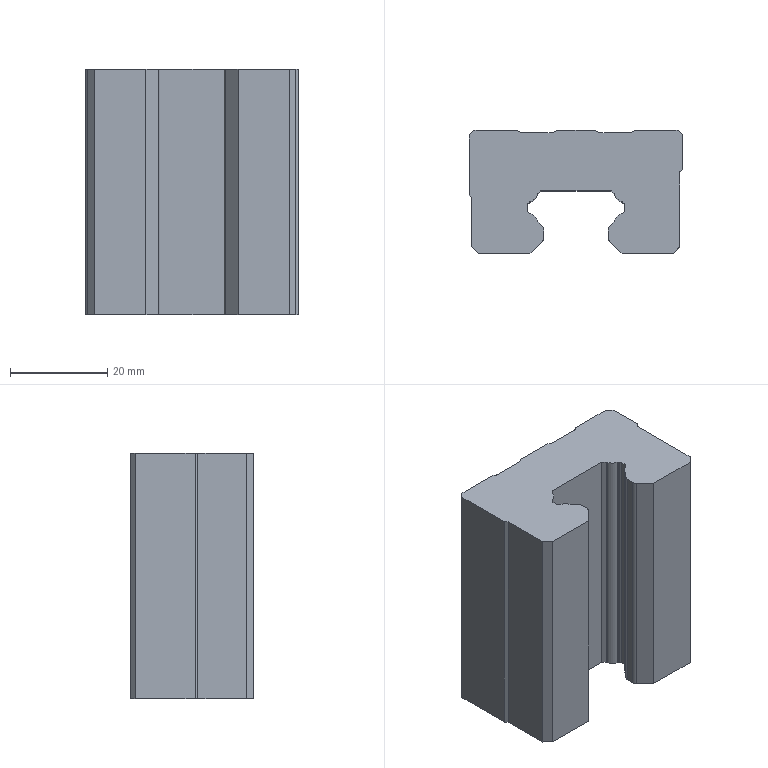Part | STEP file | PART3A^SUB1AA_P-008243 | 1 solid | 78 faces | box 44 x 25.4 x 50.5 mm | volume 44203 mm3 | plane 46 | cylinder 32 | commonest cylinder face diameters 1 x12 2 x8 4.134 x8 4.06 x4